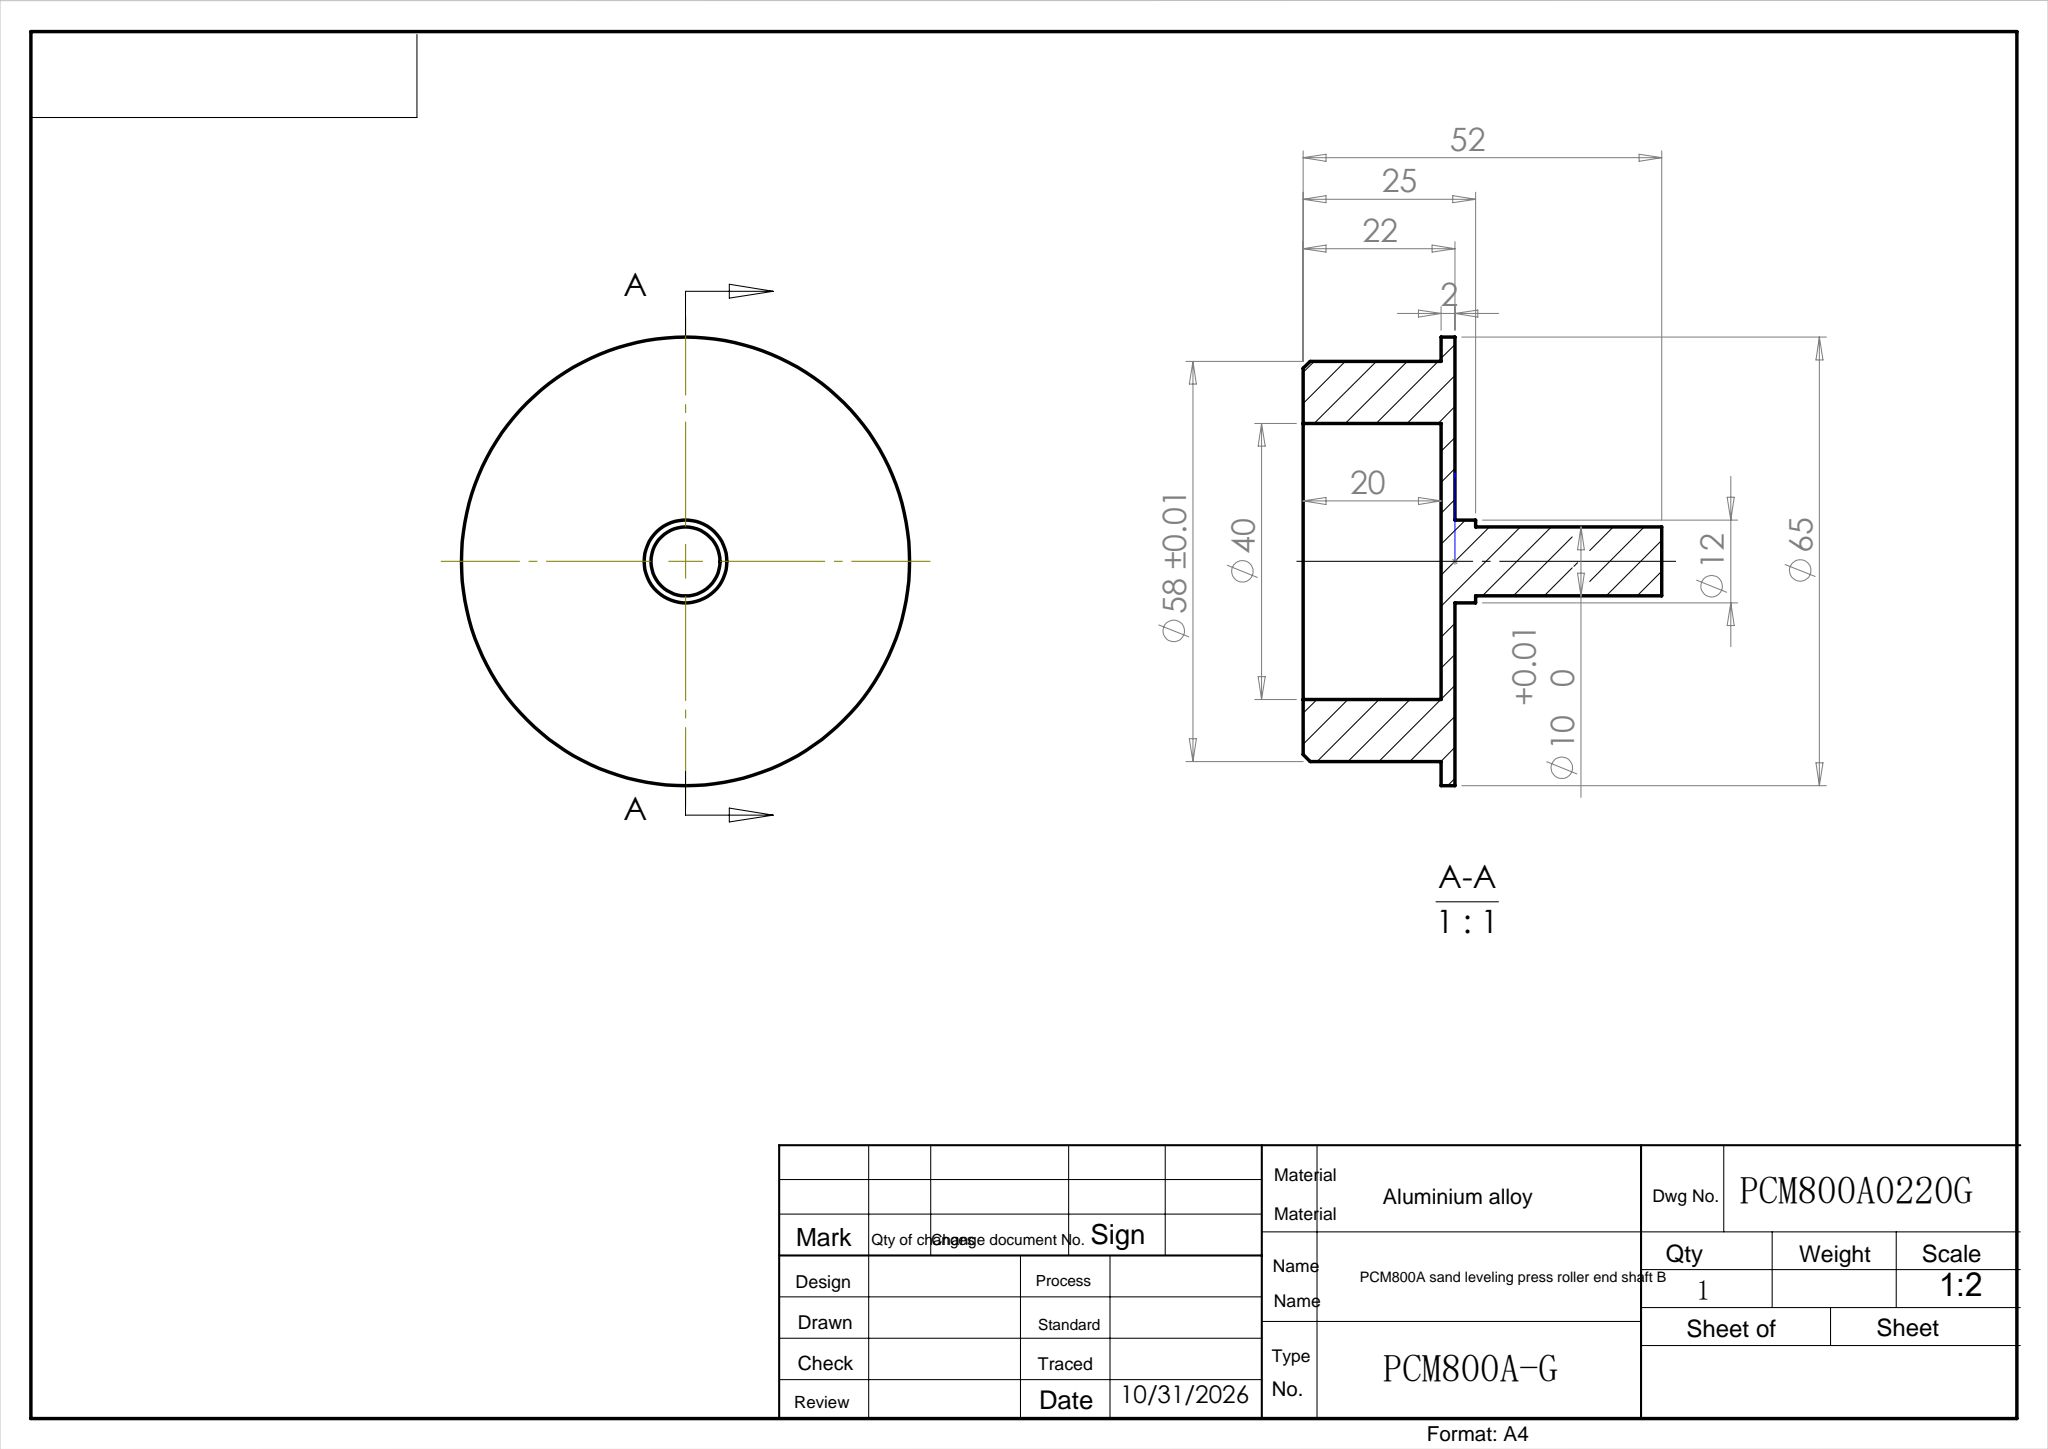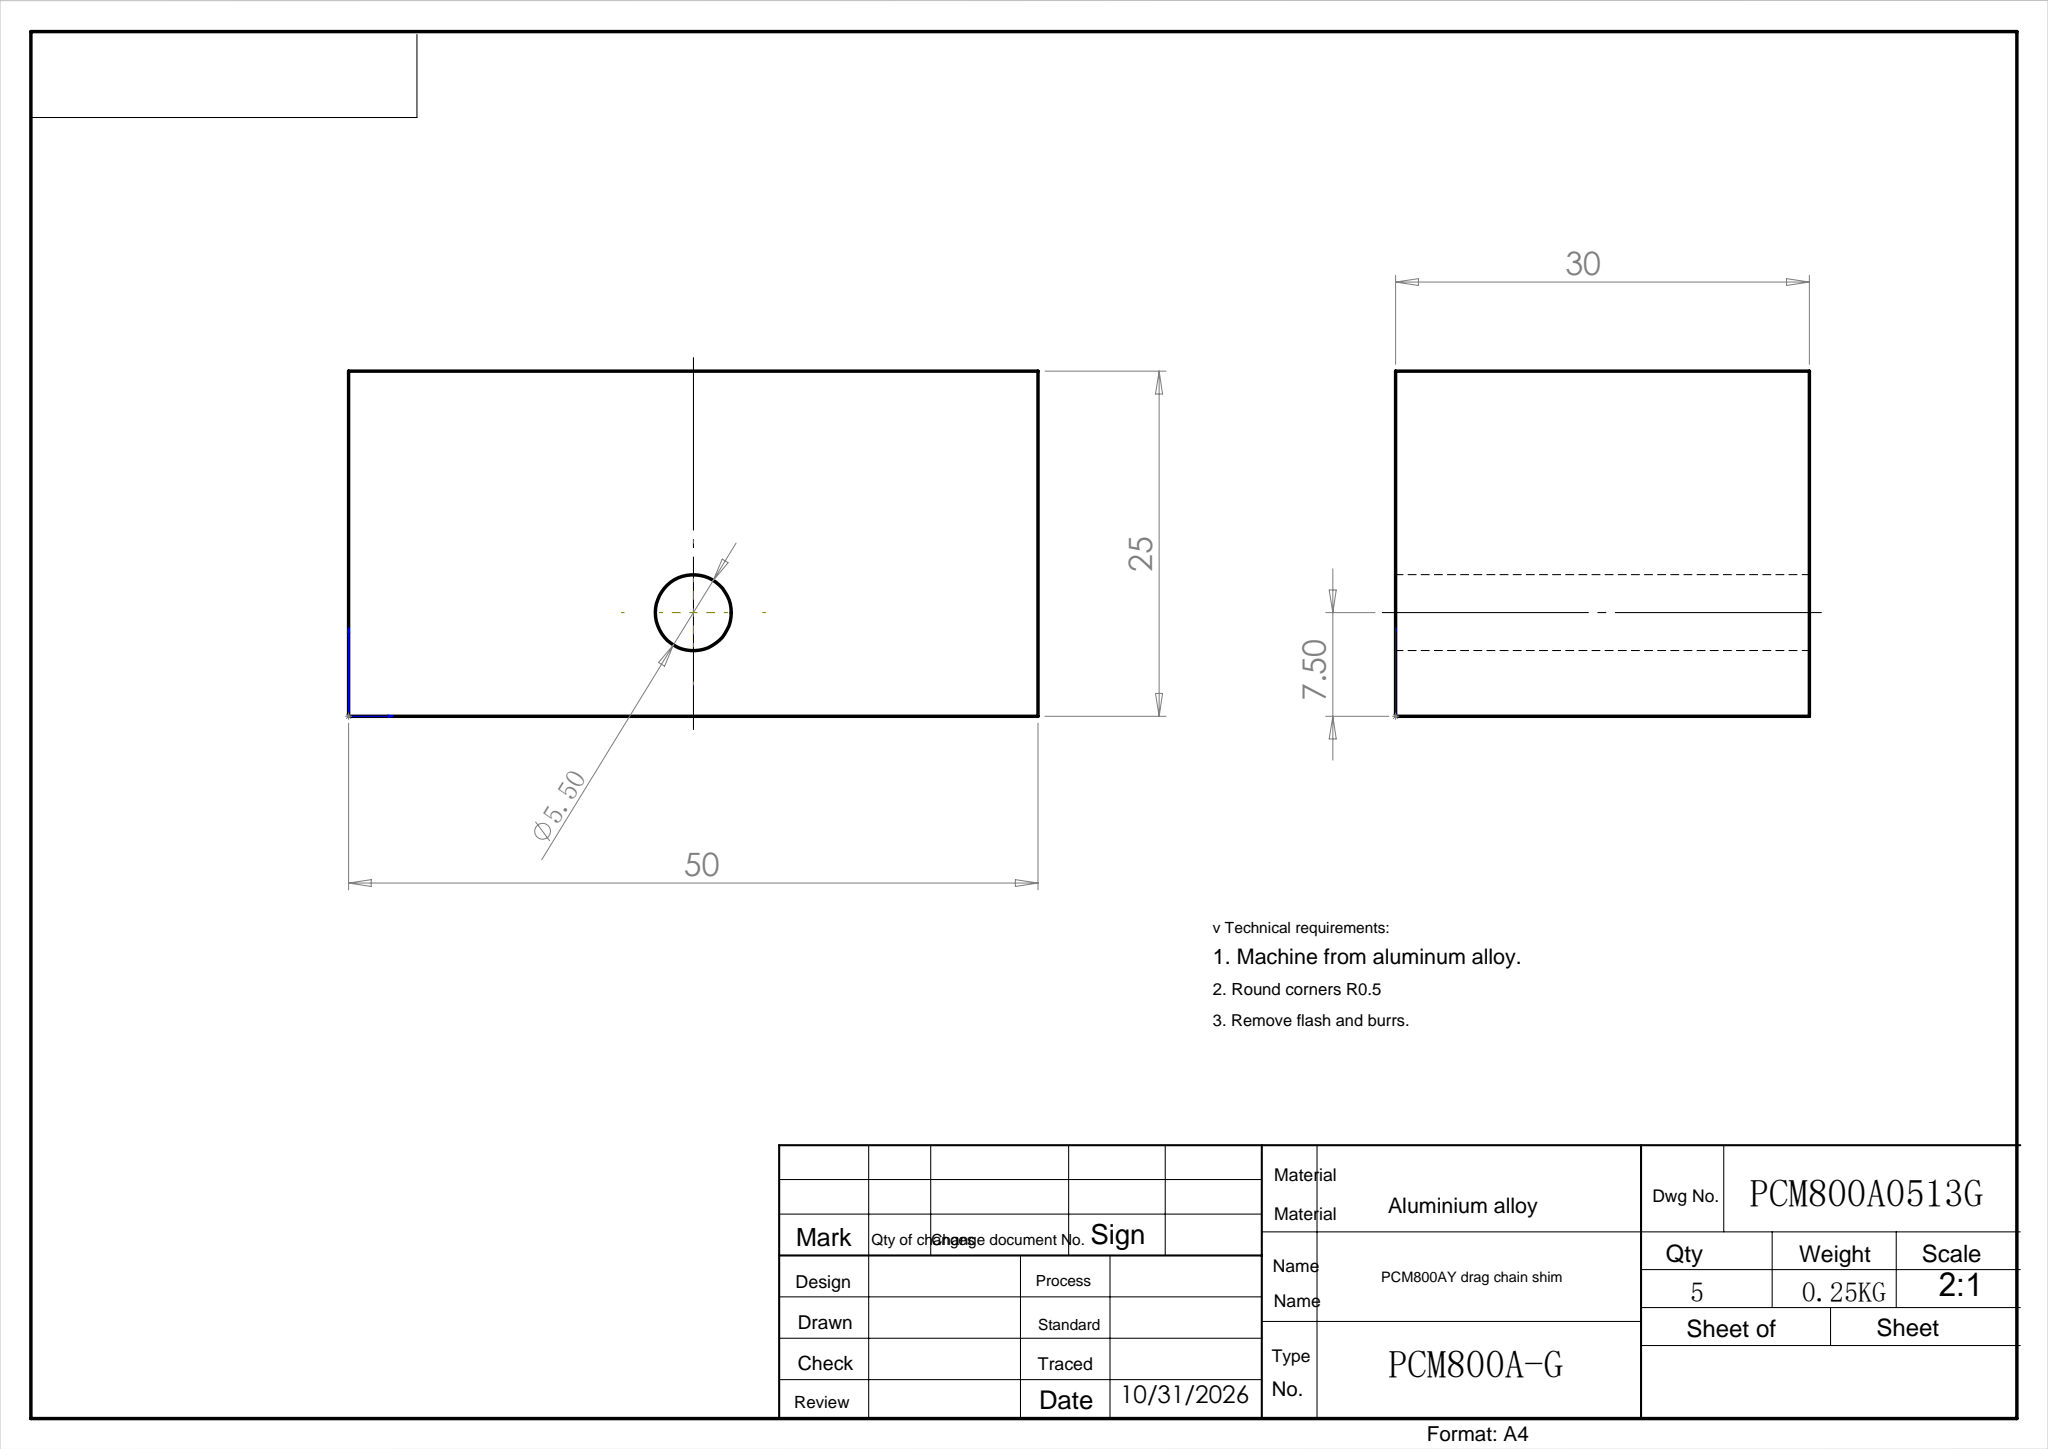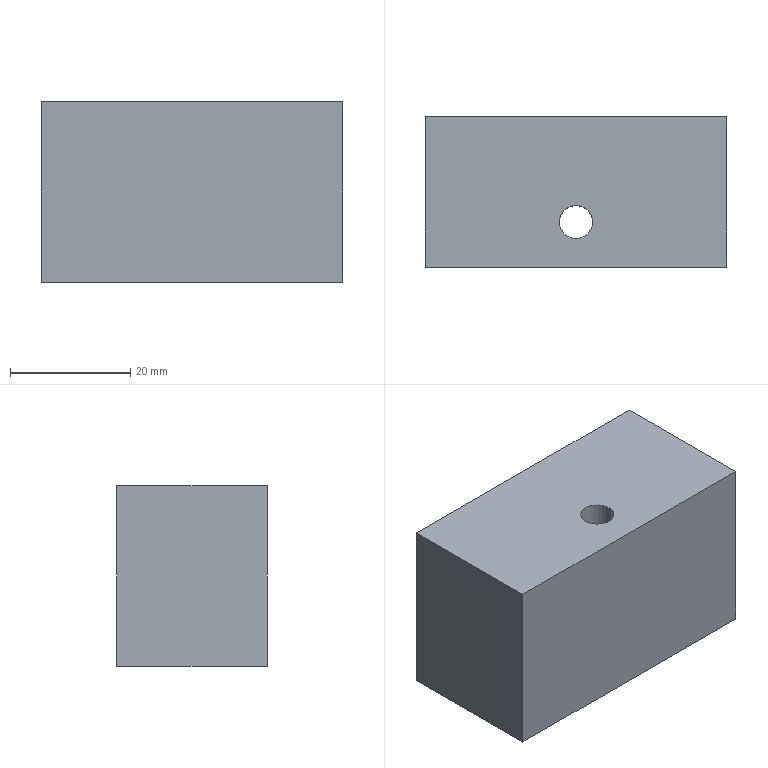Part | SolidWorks | features Extrusion 1, ICE 1 | 1 solid | 8 faces | box 50 x 25 x 30 mm | volume 36787 mm3 | plane 6 | cylinder 2 | commonest cylinder face diameters 5.5 x2
STEP:
#1=CARTESIAN_POINT('',(27.75,7.5,0.));
#2=VERTEX_POINT('',#1);
#3=CARTESIAN_POINT('',(22.25,7.5,0.));
#4=VERTEX_POINT('',#3);
#5=CARTESIAN_POINT('',(25.,7.5,0.));
#6=DIRECTION('',(0.,0.,-1.));
#7=DIRECTION('',(-1.,0.,0.));
#8=AXIS2_PLACEMENT_3D('',#5,#6,#7);
#9=CIRCLE('',#8,2.75);
#10=EDGE_CURVE('',#2,#4,#9,.T.);
#11=ORIENTED_EDGE('',*,*,#10,.T.);
#12=CARTESIAN_POINT('',(22.25,7.5,30.));
#13=VERTEX_POINT('',#12);
#14=CARTESIAN_POINT('',(22.25,7.5,-7.));
#15=DIRECTION('',(0.,0.,1.));
#16=VECTOR('',#15,1000.);
#17=LINE('',#14,#16);
#18=EDGE_CURVE('',#4,#13,#17,.T.);
#19=ORIENTED_EDGE('',*,*,#18,.T.);
#20=CARTESIAN_POINT('',(27.75,7.5,30.));
#21=VERTEX_POINT('',#20);
#22=CARTESIAN_POINT('',(25.,7.5,30.));
#23=DIRECTION('',(0.,0.,1.));
#24=DIRECTION('',(1.,0.,0.));
#25=AXIS2_PLACEMENT_3D('',#22,#23,#24);
#26=CIRCLE('',#25,2.75);
#27=EDGE_CURVE('',#13,#21,#26,.T.);
#28=ORIENTED_EDGE('',*,*,#27,.T.);
#29=CARTESIAN_POINT('',(27.75,7.5,-7.));
#30=DIRECTION('',(0.,0.,1.));
#31=VECTOR('',#30,1000.);
#32=LINE('',#29,#31);
#33=EDGE_CURVE('',#2,#21,#32,.T.);
#34=ORIENTED_EDGE('',*,*,#33,.F.);
#35=EDGE_LOOP('',(#11,#19,#28,#34));
#36=FACE_OUTER_BOUND('',#35,.T.);
#37=CARTESIAN_POINT('',(25.,7.5,-7.));
#38=DIRECTION('',(0.,0.,1.));
#39=DIRECTION('',(1.,0.,0.));
#40=AXIS2_PLACEMENT_3D('',#37,#38,#39);
#41=CYLINDRICAL_SURFACE('',#40,2.75);
#42=ADVANCED_FACE('',(#36),#41,.F.);
#43=CARTESIAN_POINT('',(0.,25.,0.));
#44=VERTEX_POINT('',#43);
#45=CARTESIAN_POINT('',(0.,0.,0.));
#46=VERTEX_POINT('',#45);
#47=CARTESIAN_POINT('',(0.,0.,0.));
#48=DIRECTION('',(0.,-1.,0.));
#49=VECTOR('',#48,1000.);
#50=LINE('',#47,#49);
#51=EDGE_CURVE('',#44,#46,#50,.T.);
#52=ORIENTED_EDGE('',*,*,#51,.T.);
#53=CARTESIAN_POINT('',(0.,0.,30.));
#54=VERTEX_POINT('',#53);
#55=CARTESIAN_POINT('',(0.,0.,30.));
#56=DIRECTION('',(0.,0.,-1.));
#57=VECTOR('',#56,1000.);
#58=LINE('',#55,#57);
#59=EDGE_CURVE('',#54,#46,#58,.T.);
#60=ORIENTED_EDGE('',*,*,#59,.F.);
#61=CARTESIAN_POINT('',(0.,25.,30.));
#62=VERTEX_POINT('',#61);
#63=CARTESIAN_POINT('',(0.,0.,30.));
#64=DIRECTION('',(0.,-1.,0.));
#65=VECTOR('',#64,1000.);
#66=LINE('',#63,#65);
#67=EDGE_CURVE('',#62,#54,#66,.T.);
#68=ORIENTED_EDGE('',*,*,#67,.F.);
#69=CARTESIAN_POINT('',(0.,25.,30.));
#70=DIRECTION('',(0.,0.,-1.));
#71=VECTOR('',#70,1000.);
#72=LINE('',#69,#71);
#73=EDGE_CURVE('',#62,#44,#72,.T.);
#74=ORIENTED_EDGE('',*,*,#73,.T.);
#75=EDGE_LOOP('',(#52,#60,#68,#74));
#76=FACE_OUTER_BOUND('',#75,.T.);
#77=CARTESIAN_POINT('',(0.,0.,30.));
#78=DIRECTION('',(1.,0.,0.));
#79=DIRECTION('',(0.,0.,-1.));
#80=AXIS2_PLACEMENT_3D('',#77,#78,#79);
#81=PLANE('',#80);
#82=ADVANCED_FACE('',(#76),#81,.F.);
#83=CARTESIAN_POINT('',(50.,0.,0.));
#84=VERTEX_POINT('',#83);
#85=CARTESIAN_POINT('',(0.,0.,0.));
#86=DIRECTION('',(1.,0.,0.));
#87=VECTOR('',#86,1000.);
#88=LINE('',#85,#87);
#89=EDGE_CURVE('',#46,#84,#88,.T.);
#90=ORIENTED_EDGE('',*,*,#89,.T.);
#91=CARTESIAN_POINT('',(50.,0.,30.));
#92=VERTEX_POINT('',#91);
#93=CARTESIAN_POINT('',(50.,0.,30.));
#94=DIRECTION('',(0.,0.,-1.));
#95=VECTOR('',#94,1000.);
#96=LINE('',#93,#95);
#97=EDGE_CURVE('',#92,#84,#96,.T.);
#98=ORIENTED_EDGE('',*,*,#97,.F.);
#99=CARTESIAN_POINT('',(0.,0.,30.));
#100=DIRECTION('',(1.,0.,0.));
#101=VECTOR('',#100,1000.);
#102=LINE('',#99,#101);
#103=EDGE_CURVE('',#54,#92,#102,.T.);
#104=ORIENTED_EDGE('',*,*,#103,.F.);
#105=ORIENTED_EDGE('',*,*,#59,.T.);
#106=EDGE_LOOP('',(#90,#98,#104,#105));
#107=FACE_OUTER_BOUND('',#106,.T.);
#108=CARTESIAN_POINT('',(0.,0.,30.));
#109=DIRECTION('',(0.,1.,0.));
#110=DIRECTION('',(0.,0.,1.));
#111=AXIS2_PLACEMENT_3D('',#108,#109,#110);
#112=PLANE('',#111);
#113=ADVANCED_FACE('',(#107),#112,.F.);
#114=CARTESIAN_POINT('',(50.,25.,0.));
#115=VERTEX_POINT('',#114);
#116=CARTESIAN_POINT('',(50.,0.,0.));
#117=DIRECTION('',(0.,1.,0.));
#118=VECTOR('',#117,1000.);
#119=LINE('',#116,#118);
#120=EDGE_CURVE('',#84,#115,#119,.T.);
#121=ORIENTED_EDGE('',*,*,#120,.T.);
#122=CARTESIAN_POINT('',(50.,25.,30.));
#123=VERTEX_POINT('',#122);
#124=CARTESIAN_POINT('',(50.,25.,30.));
#125=DIRECTION('',(0.,0.,-1.));
#126=VECTOR('',#125,1000.);
#127=LINE('',#124,#126);
#128=EDGE_CURVE('',#123,#115,#127,.T.);
#129=ORIENTED_EDGE('',*,*,#128,.F.);
#130=CARTESIAN_POINT('',(50.,0.,30.));
#131=DIRECTION('',(0.,1.,0.));
#132=VECTOR('',#131,1000.);
#133=LINE('',#130,#132);
#134=EDGE_CURVE('',#92,#123,#133,.T.);
#135=ORIENTED_EDGE('',*,*,#134,.F.);
#136=ORIENTED_EDGE('',*,*,#97,.T.);
#137=EDGE_LOOP('',(#121,#129,#135,#136));
#138=FACE_OUTER_BOUND('',#137,.T.);
#139=CARTESIAN_POINT('',(50.,0.,30.));
#140=DIRECTION('',(-1.,0.,0.));
#141=DIRECTION('',(0.,0.,1.));
#142=AXIS2_PLACEMENT_3D('',#139,#140,#141);
#143=PLANE('',#142);
#144=ADVANCED_FACE('',(#138),#143,.F.);
#145=CARTESIAN_POINT('',(0.,25.,0.));
#146=DIRECTION('',(-1.,0.,0.));
#147=VECTOR('',#146,1000.);
#148=LINE('',#145,#147);
#149=EDGE_CURVE('',#115,#44,#148,.T.);
#150=ORIENTED_EDGE('',*,*,#149,.T.);
#151=ORIENTED_EDGE('',*,*,#73,.F.);
#152=CARTESIAN_POINT('',(0.,25.,30.));
#153=DIRECTION('',(-1.,0.,0.));
#154=VECTOR('',#153,1000.);
#155=LINE('',#152,#154);
#156=EDGE_CURVE('',#123,#62,#155,.T.);
#157=ORIENTED_EDGE('',*,*,#156,.F.);
#158=ORIENTED_EDGE('',*,*,#128,.T.);
#159=EDGE_LOOP('',(#150,#151,#157,#158));
#160=FACE_OUTER_BOUND('',#159,.T.);
#161=CARTESIAN_POINT('',(0.,25.,30.));
#162=DIRECTION('',(0.,-1.,0.));
#163=DIRECTION('',(0.,0.,-1.));
#164=AXIS2_PLACEMENT_3D('',#161,#162,#163);
#165=PLANE('',#164);
#166=ADVANCED_FACE('',(#160),#165,.F.);
#167=CARTESIAN_POINT('',(25.,7.5,30.));
#168=DIRECTION('',(0.,0.,1.));
#169=DIRECTION('',(1.,0.,0.));
#170=AXIS2_PLACEMENT_3D('',#167,#168,#169);
#171=CIRCLE('',#170,2.75);
#172=EDGE_CURVE('',#21,#13,#171,.T.);
#173=ORIENTED_EDGE('',*,*,#172,.F.);
#174=ORIENTED_EDGE('',*,*,#27,.F.);
#175=EDGE_LOOP('',(#173,#174));
#176=FACE_BOUND('',#175,.T.);
#177=ORIENTED_EDGE('',*,*,#67,.T.);
#178=ORIENTED_EDGE('',*,*,#103,.T.);
#179=ORIENTED_EDGE('',*,*,#134,.T.);
#180=ORIENTED_EDGE('',*,*,#156,.T.);
#181=EDGE_LOOP('',(#177,#178,#179,#180));
#182=FACE_OUTER_BOUND('',#181,.T.);
#183=CARTESIAN_POINT('',(0.,25.,30.));
#184=DIRECTION('',(0.,0.,-1.));
#185=DIRECTION('',(-1.,0.,0.));
#186=AXIS2_PLACEMENT_3D('',#183,#184,#185);
#187=PLANE('',#186);
#188=ADVANCED_FACE('',(#176,#182),#187,.F.);
#189=ORIENTED_EDGE('',*,*,#10,.F.);
#190=CARTESIAN_POINT('',(25.,7.5,0.));
#191=DIRECTION('',(0.,0.,-1.));
#192=DIRECTION('',(-1.,0.,0.));
#193=AXIS2_PLACEMENT_3D('',#190,#191,#192);
#194=CIRCLE('',#193,2.75);
#195=EDGE_CURVE('',#4,#2,#194,.T.);
#196=ORIENTED_EDGE('',*,*,#195,.F.);
#197=EDGE_LOOP('',(#189,#196));
#198=FACE_BOUND('',#197,.T.);
#199=ORIENTED_EDGE('',*,*,#51,.F.);
#200=ORIENTED_EDGE('',*,*,#149,.F.);
#201=ORIENTED_EDGE('',*,*,#120,.F.);
#202=ORIENTED_EDGE('',*,*,#89,.F.);
#203=EDGE_LOOP('',(#199,#200,#201,#202));
#204=FACE_OUTER_BOUND('',#203,.T.);
#205=CARTESIAN_POINT('',(0.,25.,0.));
#206=DIRECTION('',(0.,0.,-1.));
#207=DIRECTION('',(-1.,0.,0.));
#208=AXIS2_PLACEMENT_3D('',#205,#206,#207);
#209=PLANE('',#208);
#210=ADVANCED_FACE('',(#198,#204),#209,.T.);
#211=ORIENTED_EDGE('',*,*,#18,.F.);
#212=ORIENTED_EDGE('',*,*,#195,.T.);
#213=ORIENTED_EDGE('',*,*,#33,.T.);
#214=ORIENTED_EDGE('',*,*,#172,.T.);
#215=EDGE_LOOP('',(#211,#212,#213,#214));
#216=FACE_OUTER_BOUND('',#215,.T.);
#217=CARTESIAN_POINT('',(25.,7.5,-7.));
#218=DIRECTION('',(0.,0.,1.));
#219=DIRECTION('',(1.,0.,0.));
#220=AXIS2_PLACEMENT_3D('',#217,#218,#219);
#221=CYLINDRICAL_SURFACE('',#220,2.75);
#222=ADVANCED_FACE('',(#216),#221,.F.);
#223=CLOSED_SHELL('',(#42,#82,#113,#144,#166,#188,#210,#222));
#224=MANIFOLD_SOLID_BREP('',#223);
#225=CARTESIAN_POINT('',(0.,0.,0.));
#226=DIRECTION('',(0.,0.,1.));
#227=DIRECTION('',(1.,0.,0.));
#228=AXIS2_PLACEMENT_3D('',#225,#226,#227);
#229=(LENGTH_UNIT()NAMED_UNIT(*)SI_UNIT(.MILLI.,.METRE.));
#230=UNCERTAINTY_MEASURE_WITH_UNIT(LENGTH_MEASURE(0.00001),#229,'','');
#231=(NAMED_UNIT(*)PLANE_ANGLE_UNIT()SI_UNIT($,.RADIAN.));
#232=(NAMED_UNIT(*)SI_UNIT($,.STERADIAN.)SOLID_ANGLE_UNIT());
#233=(GEOMETRIC_REPRESENTATION_CONTEXT(3)GLOBAL_UNCERTAINTY_ASSIGNED_CONTEXT((#230))GLOBAL_UNIT_ASSIGNED_CONTEXT((#229,#231,#232))REPRESENTATION_CONTEXT('',''));
#234=ADVANCED_BREP_SHAPE_REPRESENTATION('',(#224,#228),#233);